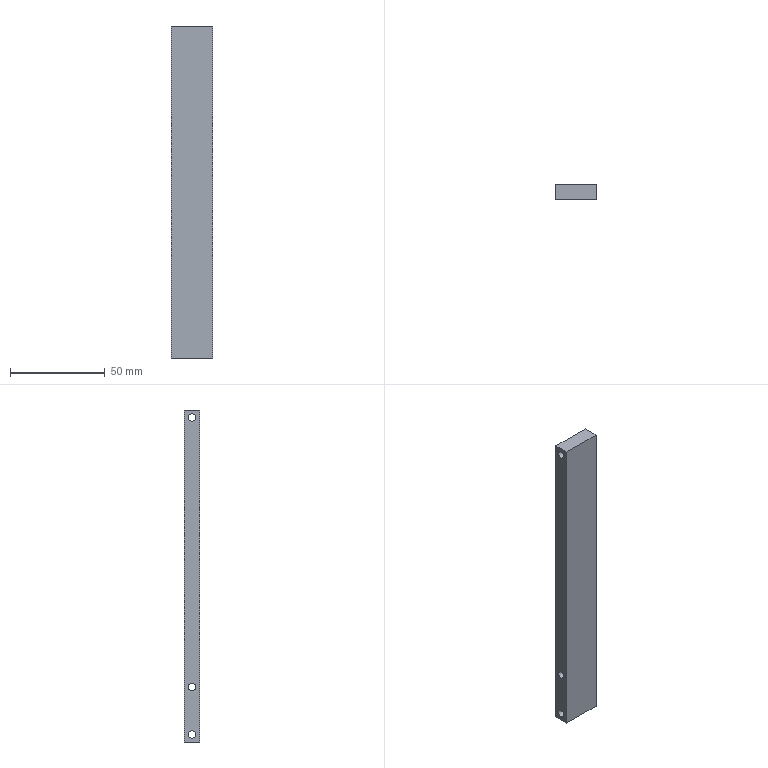Part | SolidWorks | features Extrusion 1, ICE 1 | 1 solid | 12 faces | box 22 x 8 x 175 mm | volume 29971 mm3 | cylinder 6 | plane 6 | commonest cylinder face diameters 4 x6
STEP:
#1=CARTESIAN_POINT('',(0.,4.,31.));
#2=VERTEX_POINT('',#1);
#3=CARTESIAN_POINT('',(0.,4.,27.));
#4=VERTEX_POINT('',#3);
#5=CARTESIAN_POINT('',(0.,4.,29.));
#6=DIRECTION('',(1.,0.,0.));
#7=DIRECTION('',(0.,0.,-1.));
#8=AXIS2_PLACEMENT_3D('',#5,#6,#7);
#9=CIRCLE('',#8,2.);
#10=EDGE_CURVE('',#2,#4,#9,.T.);
#11=ORIENTED_EDGE('',*,*,#10,.F.);
#12=CARTESIAN_POINT('',(22.,4.,31.));
#13=VERTEX_POINT('',#12);
#14=CARTESIAN_POINT('',(0.,4.,31.));
#15=DIRECTION('',(1.,0.,0.));
#16=VECTOR('',#15,1000.);
#17=LINE('',#14,#16);
#18=EDGE_CURVE('',#2,#13,#17,.T.);
#19=ORIENTED_EDGE('',*,*,#18,.T.);
#20=CARTESIAN_POINT('',(22.,4.,27.));
#21=VERTEX_POINT('',#20);
#22=CARTESIAN_POINT('',(22.,4.,29.));
#23=DIRECTION('',(1.,0.,0.));
#24=DIRECTION('',(0.,0.,-1.));
#25=AXIS2_PLACEMENT_3D('',#22,#23,#24);
#26=CIRCLE('',#25,2.);
#27=EDGE_CURVE('',#13,#21,#26,.T.);
#28=ORIENTED_EDGE('',*,*,#27,.T.);
#29=CARTESIAN_POINT('',(0.,4.,27.));
#30=DIRECTION('',(1.,0.,0.));
#31=VECTOR('',#30,1000.);
#32=LINE('',#29,#31);
#33=EDGE_CURVE('',#4,#21,#32,.T.);
#34=ORIENTED_EDGE('',*,*,#33,.F.);
#35=EDGE_LOOP('',(#11,#19,#28,#34));
#36=FACE_OUTER_BOUND('',#35,.T.);
#37=CARTESIAN_POINT('',(0.,4.,29.));
#38=DIRECTION('',(1.,0.,0.));
#39=DIRECTION('',(0.,0.,-1.));
#40=AXIS2_PLACEMENT_3D('',#37,#38,#39);
#41=CYLINDRICAL_SURFACE('',#40,2.);
#42=ADVANCED_FACE('',(#36),#41,.F.);
#43=CARTESIAN_POINT('',(0.,4.,173.));
#44=VERTEX_POINT('',#43);
#45=CARTESIAN_POINT('',(0.,4.,169.));
#46=VERTEX_POINT('',#45);
#47=CARTESIAN_POINT('',(0.,4.,171.));
#48=DIRECTION('',(1.,0.,0.));
#49=DIRECTION('',(0.,0.,-1.));
#50=AXIS2_PLACEMENT_3D('',#47,#48,#49);
#51=CIRCLE('',#50,2.);
#52=EDGE_CURVE('',#44,#46,#51,.T.);
#53=ORIENTED_EDGE('',*,*,#52,.F.);
#54=CARTESIAN_POINT('',(22.,4.,173.));
#55=VERTEX_POINT('',#54);
#56=CARTESIAN_POINT('',(0.,4.,173.));
#57=DIRECTION('',(1.,0.,0.));
#58=VECTOR('',#57,1000.);
#59=LINE('',#56,#58);
#60=EDGE_CURVE('',#44,#55,#59,.T.);
#61=ORIENTED_EDGE('',*,*,#60,.T.);
#62=CARTESIAN_POINT('',(22.,4.,169.));
#63=VERTEX_POINT('',#62);
#64=CARTESIAN_POINT('',(22.,4.,171.));
#65=DIRECTION('',(1.,0.,0.));
#66=DIRECTION('',(0.,0.,-1.));
#67=AXIS2_PLACEMENT_3D('',#64,#65,#66);
#68=CIRCLE('',#67,2.);
#69=EDGE_CURVE('',#55,#63,#68,.T.);
#70=ORIENTED_EDGE('',*,*,#69,.T.);
#71=CARTESIAN_POINT('',(0.,4.,169.));
#72=DIRECTION('',(1.,0.,0.));
#73=VECTOR('',#72,1000.);
#74=LINE('',#71,#73);
#75=EDGE_CURVE('',#46,#63,#74,.T.);
#76=ORIENTED_EDGE('',*,*,#75,.F.);
#77=EDGE_LOOP('',(#53,#61,#70,#76));
#78=FACE_OUTER_BOUND('',#77,.T.);
#79=CARTESIAN_POINT('',(0.,4.,171.));
#80=DIRECTION('',(1.,0.,0.));
#81=DIRECTION('',(0.,0.,-1.));
#82=AXIS2_PLACEMENT_3D('',#79,#80,#81);
#83=CYLINDRICAL_SURFACE('',#82,2.);
#84=ADVANCED_FACE('',(#78),#83,.F.);
#85=CARTESIAN_POINT('',(0.,4.,6.));
#86=VERTEX_POINT('',#85);
#87=CARTESIAN_POINT('',(0.,4.,2.));
#88=VERTEX_POINT('',#87);
#89=CARTESIAN_POINT('',(0.,4.,4.));
#90=DIRECTION('',(1.,0.,0.));
#91=DIRECTION('',(0.,0.,-1.));
#92=AXIS2_PLACEMENT_3D('',#89,#90,#91);
#93=CIRCLE('',#92,2.);
#94=EDGE_CURVE('',#86,#88,#93,.T.);
#95=ORIENTED_EDGE('',*,*,#94,.F.);
#96=CARTESIAN_POINT('',(22.,4.,6.));
#97=VERTEX_POINT('',#96);
#98=CARTESIAN_POINT('',(0.,4.,6.));
#99=DIRECTION('',(1.,0.,0.));
#100=VECTOR('',#99,1000.);
#101=LINE('',#98,#100);
#102=EDGE_CURVE('',#86,#97,#101,.T.);
#103=ORIENTED_EDGE('',*,*,#102,.T.);
#104=CARTESIAN_POINT('',(22.,4.,2.));
#105=VERTEX_POINT('',#104);
#106=CARTESIAN_POINT('',(22.,4.,4.));
#107=DIRECTION('',(1.,0.,0.));
#108=DIRECTION('',(0.,0.,-1.));
#109=AXIS2_PLACEMENT_3D('',#106,#107,#108);
#110=CIRCLE('',#109,2.);
#111=EDGE_CURVE('',#97,#105,#110,.T.);
#112=ORIENTED_EDGE('',*,*,#111,.T.);
#113=CARTESIAN_POINT('',(0.,4.,2.));
#114=DIRECTION('',(1.,0.,0.));
#115=VECTOR('',#114,1000.);
#116=LINE('',#113,#115);
#117=EDGE_CURVE('',#88,#105,#116,.T.);
#118=ORIENTED_EDGE('',*,*,#117,.F.);
#119=EDGE_LOOP('',(#95,#103,#112,#118));
#120=FACE_OUTER_BOUND('',#119,.T.);
#121=CARTESIAN_POINT('',(0.,4.,4.));
#122=DIRECTION('',(1.,0.,0.));
#123=DIRECTION('',(0.,0.,-1.));
#124=AXIS2_PLACEMENT_3D('',#121,#122,#123);
#125=CYLINDRICAL_SURFACE('',#124,2.);
#126=ADVANCED_FACE('',(#120),#125,.F.);
#127=CARTESIAN_POINT('',(0.,4.,29.));
#128=DIRECTION('',(1.,0.,0.));
#129=DIRECTION('',(0.,0.,-1.));
#130=AXIS2_PLACEMENT_3D('',#127,#128,#129);
#131=CIRCLE('',#130,2.);
#132=EDGE_CURVE('',#4,#2,#131,.T.);
#133=ORIENTED_EDGE('',*,*,#132,.T.);
#134=ORIENTED_EDGE('',*,*,#10,.T.);
#135=EDGE_LOOP('',(#133,#134));
#136=FACE_BOUND('',#135,.T.);
#137=CARTESIAN_POINT('',(0.,4.,171.));
#138=DIRECTION('',(1.,0.,0.));
#139=DIRECTION('',(0.,0.,-1.));
#140=AXIS2_PLACEMENT_3D('',#137,#138,#139);
#141=CIRCLE('',#140,2.);
#142=EDGE_CURVE('',#46,#44,#141,.T.);
#143=ORIENTED_EDGE('',*,*,#142,.T.);
#144=ORIENTED_EDGE('',*,*,#52,.T.);
#145=EDGE_LOOP('',(#143,#144));
#146=FACE_BOUND('',#145,.T.);
#147=CARTESIAN_POINT('',(0.,4.,4.));
#148=DIRECTION('',(1.,0.,0.));
#149=DIRECTION('',(0.,0.,-1.));
#150=AXIS2_PLACEMENT_3D('',#147,#148,#149);
#151=CIRCLE('',#150,2.);
#152=EDGE_CURVE('',#88,#86,#151,.T.);
#153=ORIENTED_EDGE('',*,*,#152,.T.);
#154=ORIENTED_EDGE('',*,*,#94,.T.);
#155=EDGE_LOOP('',(#153,#154));
#156=FACE_BOUND('',#155,.T.);
#157=CARTESIAN_POINT('',(0.,8.,0.));
#158=VERTEX_POINT('',#157);
#159=CARTESIAN_POINT('',(0.,0.,0.));
#160=VERTEX_POINT('',#159);
#161=CARTESIAN_POINT('',(0.,0.,0.));
#162=DIRECTION('',(0.,-1.,0.));
#163=VECTOR('',#162,1000.);
#164=LINE('',#161,#163);
#165=EDGE_CURVE('',#158,#160,#164,.T.);
#166=ORIENTED_EDGE('',*,*,#165,.T.);
#167=CARTESIAN_POINT('',(0.,0.,175.));
#168=VERTEX_POINT('',#167);
#169=CARTESIAN_POINT('',(0.,0.,175.));
#170=DIRECTION('',(0.,0.,-1.));
#171=VECTOR('',#170,1000.);
#172=LINE('',#169,#171);
#173=EDGE_CURVE('',#168,#160,#172,.T.);
#174=ORIENTED_EDGE('',*,*,#173,.F.);
#175=CARTESIAN_POINT('',(0.,8.,175.));
#176=VERTEX_POINT('',#175);
#177=CARTESIAN_POINT('',(0.,0.,175.));
#178=DIRECTION('',(0.,-1.,0.));
#179=VECTOR('',#178,1000.);
#180=LINE('',#177,#179);
#181=EDGE_CURVE('',#176,#168,#180,.T.);
#182=ORIENTED_EDGE('',*,*,#181,.F.);
#183=CARTESIAN_POINT('',(0.,8.,175.));
#184=DIRECTION('',(0.,0.,-1.));
#185=VECTOR('',#184,1000.);
#186=LINE('',#183,#185);
#187=EDGE_CURVE('',#176,#158,#186,.T.);
#188=ORIENTED_EDGE('',*,*,#187,.T.);
#189=EDGE_LOOP('',(#166,#174,#182,#188));
#190=FACE_OUTER_BOUND('',#189,.T.);
#191=CARTESIAN_POINT('',(0.,0.,175.));
#192=DIRECTION('',(1.,0.,0.));
#193=DIRECTION('',(0.,0.,-1.));
#194=AXIS2_PLACEMENT_3D('',#191,#192,#193);
#195=PLANE('',#194);
#196=ADVANCED_FACE('',(#136,#146,#156,#190),#195,.F.);
#197=CARTESIAN_POINT('',(22.,0.,0.));
#198=VERTEX_POINT('',#197);
#199=CARTESIAN_POINT('',(0.,0.,0.));
#200=DIRECTION('',(1.,0.,0.));
#201=VECTOR('',#200,1000.);
#202=LINE('',#199,#201);
#203=EDGE_CURVE('',#160,#198,#202,.T.);
#204=ORIENTED_EDGE('',*,*,#203,.T.);
#205=CARTESIAN_POINT('',(22.,0.,175.));
#206=VERTEX_POINT('',#205);
#207=CARTESIAN_POINT('',(22.,0.,175.));
#208=DIRECTION('',(0.,0.,-1.));
#209=VECTOR('',#208,1000.);
#210=LINE('',#207,#209);
#211=EDGE_CURVE('',#206,#198,#210,.T.);
#212=ORIENTED_EDGE('',*,*,#211,.F.);
#213=CARTESIAN_POINT('',(0.,0.,175.));
#214=DIRECTION('',(1.,0.,0.));
#215=VECTOR('',#214,1000.);
#216=LINE('',#213,#215);
#217=EDGE_CURVE('',#168,#206,#216,.T.);
#218=ORIENTED_EDGE('',*,*,#217,.F.);
#219=ORIENTED_EDGE('',*,*,#173,.T.);
#220=EDGE_LOOP('',(#204,#212,#218,#219));
#221=FACE_OUTER_BOUND('',#220,.T.);
#222=CARTESIAN_POINT('',(0.,0.,175.));
#223=DIRECTION('',(0.,1.,0.));
#224=DIRECTION('',(0.,0.,1.));
#225=AXIS2_PLACEMENT_3D('',#222,#223,#224);
#226=PLANE('',#225);
#227=ADVANCED_FACE('',(#221),#226,.F.);
#228=CARTESIAN_POINT('',(22.,4.,29.));
#229=DIRECTION('',(1.,0.,0.));
#230=DIRECTION('',(0.,0.,-1.));
#231=AXIS2_PLACEMENT_3D('',#228,#229,#230);
#232=CIRCLE('',#231,2.);
#233=EDGE_CURVE('',#21,#13,#232,.T.);
#234=ORIENTED_EDGE('',*,*,#233,.F.);
#235=ORIENTED_EDGE('',*,*,#27,.F.);
#236=EDGE_LOOP('',(#234,#235));
#237=FACE_BOUND('',#236,.T.);
#238=CARTESIAN_POINT('',(22.,4.,171.));
#239=DIRECTION('',(1.,0.,0.));
#240=DIRECTION('',(0.,0.,-1.));
#241=AXIS2_PLACEMENT_3D('',#238,#239,#240);
#242=CIRCLE('',#241,2.);
#243=EDGE_CURVE('',#63,#55,#242,.T.);
#244=ORIENTED_EDGE('',*,*,#243,.F.);
#245=ORIENTED_EDGE('',*,*,#69,.F.);
#246=EDGE_LOOP('',(#244,#245));
#247=FACE_BOUND('',#246,.T.);
#248=CARTESIAN_POINT('',(22.,4.,4.));
#249=DIRECTION('',(1.,0.,0.));
#250=DIRECTION('',(0.,0.,-1.));
#251=AXIS2_PLACEMENT_3D('',#248,#249,#250);
#252=CIRCLE('',#251,2.);
#253=EDGE_CURVE('',#105,#97,#252,.T.);
#254=ORIENTED_EDGE('',*,*,#253,.F.);
#255=ORIENTED_EDGE('',*,*,#111,.F.);
#256=EDGE_LOOP('',(#254,#255));
#257=FACE_BOUND('',#256,.T.);
#258=CARTESIAN_POINT('',(22.,8.,0.));
#259=VERTEX_POINT('',#258);
#260=CARTESIAN_POINT('',(22.,0.,0.));
#261=DIRECTION('',(0.,1.,0.));
#262=VECTOR('',#261,1000.);
#263=LINE('',#260,#262);
#264=EDGE_CURVE('',#198,#259,#263,.T.);
#265=ORIENTED_EDGE('',*,*,#264,.T.);
#266=CARTESIAN_POINT('',(22.,8.,175.));
#267=VERTEX_POINT('',#266);
#268=CARTESIAN_POINT('',(22.,8.,175.));
#269=DIRECTION('',(0.,0.,-1.));
#270=VECTOR('',#269,1000.);
#271=LINE('',#268,#270);
#272=EDGE_CURVE('',#267,#259,#271,.T.);
#273=ORIENTED_EDGE('',*,*,#272,.F.);
#274=CARTESIAN_POINT('',(22.,0.,175.));
#275=DIRECTION('',(0.,1.,0.));
#276=VECTOR('',#275,1000.);
#277=LINE('',#274,#276);
#278=EDGE_CURVE('',#206,#267,#277,.T.);
#279=ORIENTED_EDGE('',*,*,#278,.F.);
#280=ORIENTED_EDGE('',*,*,#211,.T.);
#281=EDGE_LOOP('',(#265,#273,#279,#280));
#282=FACE_OUTER_BOUND('',#281,.T.);
#283=CARTESIAN_POINT('',(22.,0.,175.));
#284=DIRECTION('',(-1.,0.,0.));
#285=DIRECTION('',(0.,0.,1.));
#286=AXIS2_PLACEMENT_3D('',#283,#284,#285);
#287=PLANE('',#286);
#288=ADVANCED_FACE('',(#237,#247,#257,#282),#287,.F.);
#289=CARTESIAN_POINT('',(0.,8.,0.));
#290=DIRECTION('',(-1.,0.,0.));
#291=VECTOR('',#290,1000.);
#292=LINE('',#289,#291);
#293=EDGE_CURVE('',#259,#158,#292,.T.);
#294=ORIENTED_EDGE('',*,*,#293,.T.);
#295=ORIENTED_EDGE('',*,*,#187,.F.);
#296=CARTESIAN_POINT('',(0.,8.,175.));
#297=DIRECTION('',(-1.,0.,0.));
#298=VECTOR('',#297,1000.);
#299=LINE('',#296,#298);
#300=EDGE_CURVE('',#267,#176,#299,.T.);
#301=ORIENTED_EDGE('',*,*,#300,.F.);
#302=ORIENTED_EDGE('',*,*,#272,.T.);
#303=EDGE_LOOP('',(#294,#295,#301,#302));
#304=FACE_OUTER_BOUND('',#303,.T.);
#305=CARTESIAN_POINT('',(0.,8.,175.));
#306=DIRECTION('',(0.,-1.,0.));
#307=DIRECTION('',(0.,0.,-1.));
#308=AXIS2_PLACEMENT_3D('',#305,#306,#307);
#309=PLANE('',#308);
#310=ADVANCED_FACE('',(#304),#309,.F.);
#311=ORIENTED_EDGE('',*,*,#181,.T.);
#312=ORIENTED_EDGE('',*,*,#217,.T.);
#313=ORIENTED_EDGE('',*,*,#278,.T.);
#314=ORIENTED_EDGE('',*,*,#300,.T.);
#315=EDGE_LOOP('',(#311,#312,#313,#314));
#316=FACE_OUTER_BOUND('',#315,.T.);
#317=CARTESIAN_POINT('',(0.,0.,175.));
#318=DIRECTION('',(0.,0.,-1.));
#319=DIRECTION('',(-1.,0.,0.));
#320=AXIS2_PLACEMENT_3D('',#317,#318,#319);
#321=PLANE('',#320);
#322=ADVANCED_FACE('',(#316),#321,.F.);
#323=ORIENTED_EDGE('',*,*,#165,.F.);
#324=ORIENTED_EDGE('',*,*,#293,.F.);
#325=ORIENTED_EDGE('',*,*,#264,.F.);
#326=ORIENTED_EDGE('',*,*,#203,.F.);
#327=EDGE_LOOP('',(#323,#324,#325,#326));
#328=FACE_OUTER_BOUND('',#327,.T.);
#329=CARTESIAN_POINT('',(0.,0.,0.));
#330=DIRECTION('',(0.,0.,-1.));
#331=DIRECTION('',(-1.,0.,0.));
#332=AXIS2_PLACEMENT_3D('',#329,#330,#331);
#333=PLANE('',#332);
#334=ADVANCED_FACE('',(#328),#333,.T.);
#335=ORIENTED_EDGE('',*,*,#102,.F.);
#336=ORIENTED_EDGE('',*,*,#152,.F.);
#337=ORIENTED_EDGE('',*,*,#117,.T.);
#338=ORIENTED_EDGE('',*,*,#253,.T.);
#339=EDGE_LOOP('',(#335,#336,#337,#338));
#340=FACE_OUTER_BOUND('',#339,.T.);
#341=CARTESIAN_POINT('',(0.,4.,4.));
#342=DIRECTION('',(1.,0.,0.));
#343=DIRECTION('',(0.,0.,-1.));
#344=AXIS2_PLACEMENT_3D('',#341,#342,#343);
#345=CYLINDRICAL_SURFACE('',#344,2.);
#346=ADVANCED_FACE('',(#340),#345,.F.);
#347=ORIENTED_EDGE('',*,*,#60,.F.);
#348=ORIENTED_EDGE('',*,*,#142,.F.);
#349=ORIENTED_EDGE('',*,*,#75,.T.);
#350=ORIENTED_EDGE('',*,*,#243,.T.);
#351=EDGE_LOOP('',(#347,#348,#349,#350));
#352=FACE_OUTER_BOUND('',#351,.T.);
#353=CARTESIAN_POINT('',(0.,4.,171.));
#354=DIRECTION('',(1.,0.,0.));
#355=DIRECTION('',(0.,0.,-1.));
#356=AXIS2_PLACEMENT_3D('',#353,#354,#355);
#357=CYLINDRICAL_SURFACE('',#356,2.);
#358=ADVANCED_FACE('',(#352),#357,.F.);
#359=ORIENTED_EDGE('',*,*,#18,.F.);
#360=ORIENTED_EDGE('',*,*,#132,.F.);
#361=ORIENTED_EDGE('',*,*,#33,.T.);
#362=ORIENTED_EDGE('',*,*,#233,.T.);
#363=EDGE_LOOP('',(#359,#360,#361,#362));
#364=FACE_OUTER_BOUND('',#363,.T.);
#365=CARTESIAN_POINT('',(0.,4.,29.));
#366=DIRECTION('',(1.,0.,0.));
#367=DIRECTION('',(0.,0.,-1.));
#368=AXIS2_PLACEMENT_3D('',#365,#366,#367);
#369=CYLINDRICAL_SURFACE('',#368,2.);
#370=ADVANCED_FACE('',(#364),#369,.F.);
#371=CLOSED_SHELL('',(#42,#84,#126,#196,#227,#288,#310,#322,#334,#346,#358,#370));
#372=MANIFOLD_SOLID_BREP('',#371);
#373=CARTESIAN_POINT('',(0.,0.,0.));
#374=DIRECTION('',(0.,0.,1.));
#375=DIRECTION('',(1.,0.,0.));
#376=AXIS2_PLACEMENT_3D('',#373,#374,#375);
#377=(LENGTH_UNIT()NAMED_UNIT(*)SI_UNIT(.MILLI.,.METRE.));
#378=UNCERTAINTY_MEASURE_WITH_UNIT(LENGTH_MEASURE(0.00001),#377,'','');
#379=(NAMED_UNIT(*)PLANE_ANGLE_UNIT()SI_UNIT($,.RADIAN.));
#380=(NAMED_UNIT(*)SI_UNIT($,.STERADIAN.)SOLID_ANGLE_UNIT());
#381=(GEOMETRIC_REPRESENTATION_CONTEXT(3)GLOBAL_UNCERTAINTY_ASSIGNED_CONTEXT((#378))GLOBAL_UNIT_ASSIGNED_CONTEXT((#377,#379,#380))REPRESENTATION_CONTEXT('',''));
#382=ADVANCED_BREP_SHAPE_REPRESENTATION('',(#372,#376),#381);